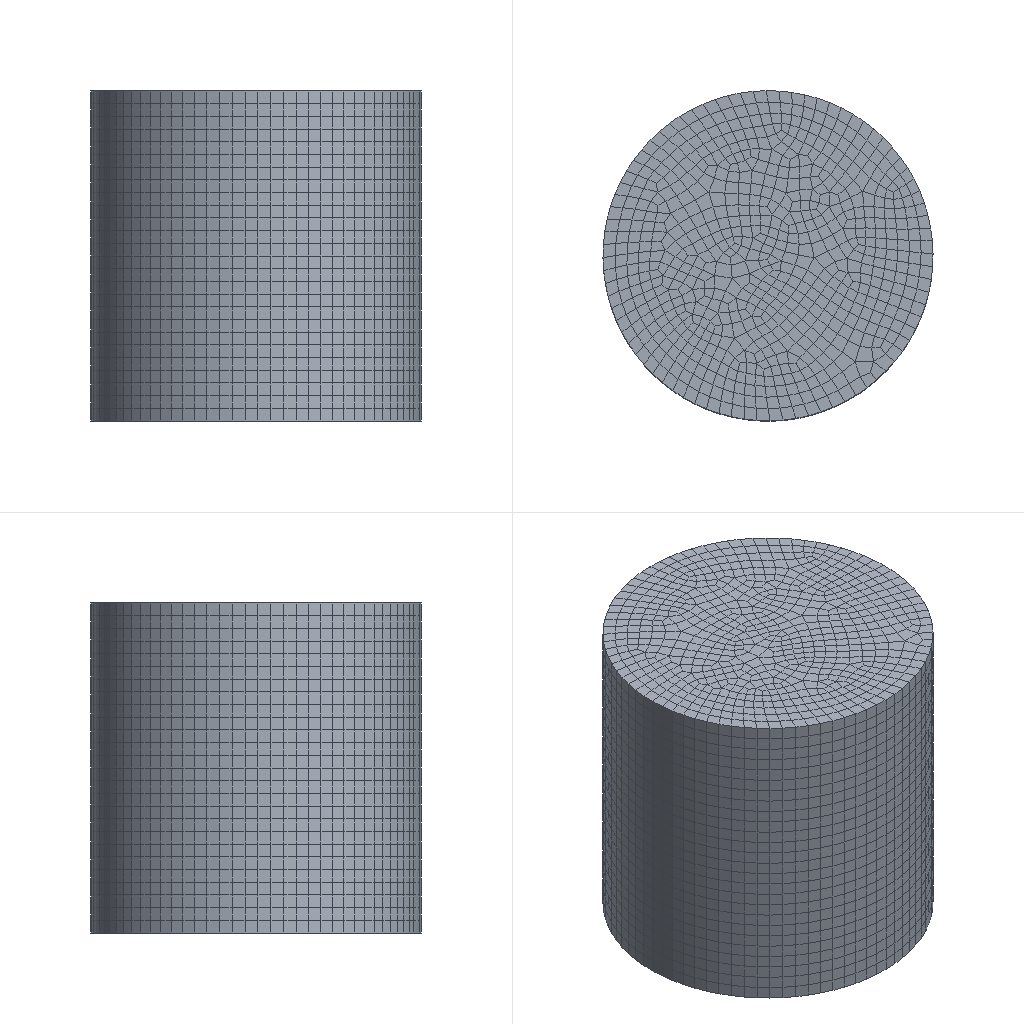Simulation study | abaqus
Set-up summary:
category,name,step,type,value,unit,region
solver,abaqus
solver,version,,,Abaqus/Explicit 2020
units,not stated in the deck,,not stated
analysis,deck,,transient,transient
load_step,Step-1,Step-1,transient
load_step,requested,,,1
mesh,nodes,,,20804
mesh,elements,,,18954
element_type,C3D8R,,solid,18252
element_type,COH3D8,,cohesive,702
load,load commands in deck,,count,2
bc,support commands in deck,,count,12
material,COH,,in results
material,MATERIAL-1,,in results
check,setup vs results,,match,"per instance, exact: element labels, types and connectivity; labels of the nodes the elements use; coordinates of those nodes at SINGLE_PRECISION in 1 of 1 instance(s)"
Abaqus input file, long lists of numbers shortened:
*Heading
** Job name: Job-2 Model name: Model-1-Copy
** Generated by: Abaqus/CAE 2020
*Preprint, echo=NO, model=NO, history=NO, contact=NO
**
** PARTS
**
*Part, name=Part-1
*Node
      1,   19.206,  -16.005,          25.
      2,   19.206,  -16.005,          50.
** (20802 more lines like these left out)
*Element, type=C3D8R
   1,  1575,  4160,  4244,  1574, 20062, 20063, 20064, 20065
   2,  4161,  1577,  1578,  4162, 20066, 20067, 20068, 20069
** (18250 more lines like these left out)
*Element, type=COH3D8
18253,    10,   335,   251,    11, 20065, 20064, 20063, 20062
18254,   253,    14,    13,   252, 20069, 20068, 20067, 20066
** (700 more lines like these left out)
*Nset, nset=Set-1, generate
     1,  20804,      1
*Elset, elset=Set-1, generate
     1,  18252,      1
*Elset, elset=CohesiveSeam-1-Elements, generate
 18253,  18954,      1
*Nset, nset=CohesiveSeam-1-TopNodes, generate
 20062,  20804,      1
*Nset, nset=CohesiveSeam-1-BottomNodes
   1,   4,   5,   6,   7,   8,   9,  10,  11,  12,  13,  14,  15,  16,  17,  18
  19,  20,  21,  22,  23,  24,  25,  26,  27,  28,  29,  30,  31,  32,  33,  34
** (45 more lines like these left out)
*Elset, elset=__PickedSurf8_S1, internal, generate
 18253,  18954,      1
*Surface, type=ELEMENT, name=_PickedSurf8, internal
__PickedSurf8_S1, S1
*Elset, elset=_CohesiveSeam-1-TopSurf_S2, internal, generate
 18253,  18954,      1
*Surface, type=ELEMENT, name=CohesiveSeam-1-TopSurf
_CohesiveSeam-1-TopSurf_S2, S2
*Elset, elset=_CohesiveSeam-1-BottomSurf_S1, internal, generate
 18253,  18954,      1
*Surface, type=ELEMENT, name=CohesiveSeam-1-BottomSurf
_CohesiveSeam-1-BottomSurf_S1, S1
** Section: Section-1
*Solid Section, elset=Set-1, material=Material-1
,
** Section: coh
*Cohesive Section, elset=CohesiveSeam-1-Elements, controls=EC-1, material=coh, response=TRACTION SEPARATION
,
*End Part
**
**
** ASSEMBLY
**
*Assembly, name=Assembly
**
*Instance, name=Part-1-1, part=Part-1
*End Instance
**
*Node
      1,           0., 1.53080845e-15,           0.
*Nset, nset=Set-1, instance=Part-1-1
    1,    3,    4,    5,    6,    7,    8,    9,   10,   11,   12,   13,   14,   15,   16,   17
   18,   19,   20,   21,   22,   23,   24,   25,   26,   27,   28,   29,   30,   31,   32,   33
** (68 more lines like these left out)
*Elset, elset=Set-1, instance=Part-1-1
  9127,  9128,  9129,  9130,  9131,  9132,  9133,  9134,  9136,  9137,  9138,  9140,  9141,  9143,  9144,  9145
  9147,  9148,  9150,  9151,  9152,  9153,  9154,  9155,  9156,  9159,  9160,  9162,  9163,  9164,  9166,  9167
** (63 more lines like these left out)
*Nset, nset=Set-2, instance=Part-1-1
     2,    83,    84,    85,    86,    87,    88,    89,    90,    91,    92,    93,    94,    95,    96,    97
    98,    99,   100,   101,   102,   103,   104,   105,   106,   107,   108,   109,   110,   111,   112,   113
** (68 more lines like these left out)
*Elset, elset=Set-2, instance=Part-1-1
    1,    2,    3,    4,    5,    6,    7,    8,   10,   11,   12,   14,   15,   17,   18,   19
   21,   22,   24,   25,   26,   27,   28,   29,   30,   33,   34,   36,   37,   38,   40,   41
** (63 more lines like these left out)
*Nset, nset=Set-3, instance=Part-1-1
    3,  162,  163,  164,  165,  166,  167,  168,  169,  170,  171,  172,  173,  174,  175,  176
  177,  178,  179,  180,  181,  182,  183,  184,  185,  186,  187,  188,  189,  190,  191,  192
** (45 more lines like these left out)
*Elset, elset=Set-3, instance=Part-1-1, generate
 17551,  18252,      1
*Nset, nset=Set-5
 1,
*Nset, nset=Set-6, instance=Part-1-1, generate
     1,  20804,      1
*Nset, nset=Set-6
 1,
*Elset, elset=Set-6, instance=Part-1-1, generate
     1,  18954,      1
*Nset, nset=m_Set-4
 1,
*Elset, elset=_Surf-2_S1, internal, instance=Part-1-1, generate
 8425,  9126,     1
*Surface, type=ELEMENT, name=Surf-2
_Surf-2_S1, S1
*Elset, elset=_s_Surf-1_S2, internal, instance=Part-1-1, generate
 17551,  18252,      1
*Surface, type=ELEMENT, name=s_Surf-1
_s_Surf-1_S2, S2
** Constraint: Constraint-1
*Coupling, constraint name=Constraint-1, ref node=m_Set-4, surface=s_Surf-1
*Kinematic
*End Assembly
**
** ELEMENT CONTROLS
**
*Section Controls, name=EC-1, ELEMENT DELETION=YES, VISCOSITY=0.01
1., 1., 1.
*Amplitude, name=Amp-1
             0.,              0.,             0.1,              1.
**
** MATERIALS
**
*Material, name=Material-1
*Conductivity
5.,
*Density
 2.7e-09,
*Elastic
32500., 0.2
*Expansion
 1e-06,
*Specific Heat
 9.7e+08,
*Concrete Damaged Plasticity
30.,   0.1,  1.16, 0.667,  0.01
*Concrete Compression Hardening
 31.839,          0.
  35.238, 0.0001688
  37.656, 0.0002734
 39.058, 0.0004092
    39.5, 0.0005746
 38.815, 0.0007747
 37.101,  0.001006
  34.823,  0.001256
 32.332,  0.001511
 29.849,  0.001767
 27.497,  0.002018
 25.334,   0.002263
 23.376,  0.002503
 21.619,  0.002736
 20.051,  0.002963
 18.651,  0.003185
 17.402,  0.003403
 16.285,  0.003616
 15.284,  0.003826
 14.385,   0.004032
 13.573,  0.004236
 12.839,  0.004438
 12.173,  0.004637
 11.567,   0.004835
  11.013,  0.005031
*Concrete Tension Stiffening
  2.09,       0.
   2.4, 8.74e-06
  2.67, 1.23e-05
  2.86, 1.81e-05
  2.94, 2.75e-05
   2.8, 4.37e-05
  2.55, 6.31e-05
   2.3, 8.27e-05
  2.07, 0.000102
  1.86,  0.00012
  1.69, 0.000137
  1.55, 0.000153
  1.42, 0.000169
  1.31, 0.000184
  1.22, 0.000198
  1.14, 0.000213
  1.07, 0.000227
  1.01,  0.00024
 0.956, 0.000254
 0.908, 0.000267
 0.864,  0.00028
 0.825, 0.000293
 0.789, 0.000306
 0.757, 0.000319
 0.727, 0.000332
*Concrete Compression Damage
        0.,          0.
 0.06977, 0.0001688
  0.1005, 0.0002734
  0.1363, 0.0004092
  0.176, 0.0005746
  0.2212, 0.0007747
  0.271,  0.001006
  0.3214,  0.001256
  0.3699,  0.001511
  0.4151,  0.001767
  0.4565,  0.002018
  0.4939,   0.002263
  0.5275,  0.002503
   0.5577,  0.002736
  0.5849,  0.002963
   0.6093,  0.003185
  0.6313,  0.003403
  0.6511,  0.003616
  0.6691,  0.003826
  0.6855,   0.004032
  0.7004,  0.004236
  0.7141,  0.004438
  0.7266,  0.004637
  0.7382,   0.004835
  0.7488,  0.005031
  0.7586,  0.005226
  0.7678,  0.005419
  0.7763,  0.005611
  0.7842,  0.005802
  0.7915,  0.005993
  0.7984,  0.006182
  0.8049,  0.006371
  0.811,  0.006559
  0.8167,  0.006747
  0.8221,  0.006933
  0.8627,  0.008781
  0.8884,   0.01061
  0.906,   0.01242
  0.9188,   0.01423
  0.9286,   0.01603
** (21 more lines like these left out)
*Concrete Tension Damage, compression recovery=0.45
     0.,       0.
 0.0544, 8.74e-06
 0.0674, 1.23e-05
 0.0893, 1.81e-05
  0.124, 2.75e-05
  0.186, 4.37e-05
  0.255, 6.31e-05
  0.321, 8.27e-05
   0.38, 0.000102
  0.431,  0.00012
  0.475, 0.000137
  0.513, 0.000153
  0.546, 0.000169
  0.575, 0.000184
  0.601, 0.000198
  0.623, 0.000213
  0.643, 0.000227
  0.661,  0.00024
  0.678, 0.000254
  0.692, 0.000267
  0.706,  0.00028
  0.718, 0.000293
  0.729, 0.000306
  0.739, 0.000319
  0.749, 0.000332
  0.757, 0.000344
  0.765, 0.000357
  0.773, 0.000369
   0.78, 0.000382
  0.787, 0.000394
  0.793, 0.000407
  0.799, 0.000419
  0.804, 0.000431
  0.809, 0.000443
  0.814, 0.000456
  0.851, 0.000577
  0.875, 0.000697
  0.892, 0.000816
  0.905, 0.000935
  0.915,  0.00105
** (31 more lines like these left out)
*Material, name=coh
*Damage Initiation, criterion=MAXS
15.,15.,15.
*Damage Evolution, type=DISPLACEMENT
 1e-11,
*Damage Stabilization
0.01
*Density
 2.7e-09,
*Elastic, type=TRACTION
20000.,20000.,20000.
**
** INTERACTION PROPERTIES
**
*Surface Interaction, name=IntProp-1
*Friction
 0.1,
*Surface Behavior, pressure-overclosure=HARD
**
** INTERACTIONS
**
** Interaction: Int-2
*Contact, op=NEW
*Contact Inclusions, ALL EXTERIOR
*Contact Property Assignment
 ,  , IntProp-1
** ----------------------------------------------------------------
**
** STEP: Step-1
**
*Step, name=Step-1, nlgeom=YES
*Dynamic, Explicit
, 0.1
*Bulk Viscosity
0.06, 1.2
** Mass Scaling: Semi-Automatic
**               Whole Model
*Fixed Mass Scaling, factor=50.
**
** BOUNDARY CONDITIONS
**
** Name: BC-1 Type: 位移/转角
*Boundary
Set-5, 1, 1
Set-5, 2, 2
Set-5, 3, 3
Set-5, 4, 4
Set-5, 5, 5
Set-5, 6, 6
** Name: BC-2 Type: 位移/转角
*Boundary, amplitude=Amp-1
Set-2, 1, 1, 6.
Set-2, 2, 2
Set-2, 3, 3
Set-2, 4, 4
Set-2, 5, 5
Set-2, 6, 6
**
** LOADS
**
** Name: Load-1   Type: Pressure
*Dsload, amplitude=Amp-1
Surf-2, P, 50.
**
** OUTPUT REQUESTS
**
*Restart, write, number interval=1, time marks=NO
**
** FIELD OUTPUT: F-Output-1
**
*Output, field, number interval=50
*Node Output
RF, RM, RT, U, V
*Element Output, directions=YES
DAMAGEC, DAMAGET, E, LE, MISES, MISESMAX, PE, PEEQ, S, SDEG, STATUS
*Contact Output
CDISP, CSTRESS
**
** HISTORY OUTPUT: H-Output-1
**
*Output, history, time interval=1e-05
*Node Output, nset=Set-5
RF1, RF2, U1, U2
*End Step
Results summary:
result,step,Step-1,completed,increments=59635 time=0.1/0.1
result,analysis,,,transient
result,last_loadstep,,,1
result,primary field,,,U
result,reaction total,,FX,9.752,model units
result,reaction total,,FY,-7.869,model units
result,reaction total,,FZ,98191.302,model units